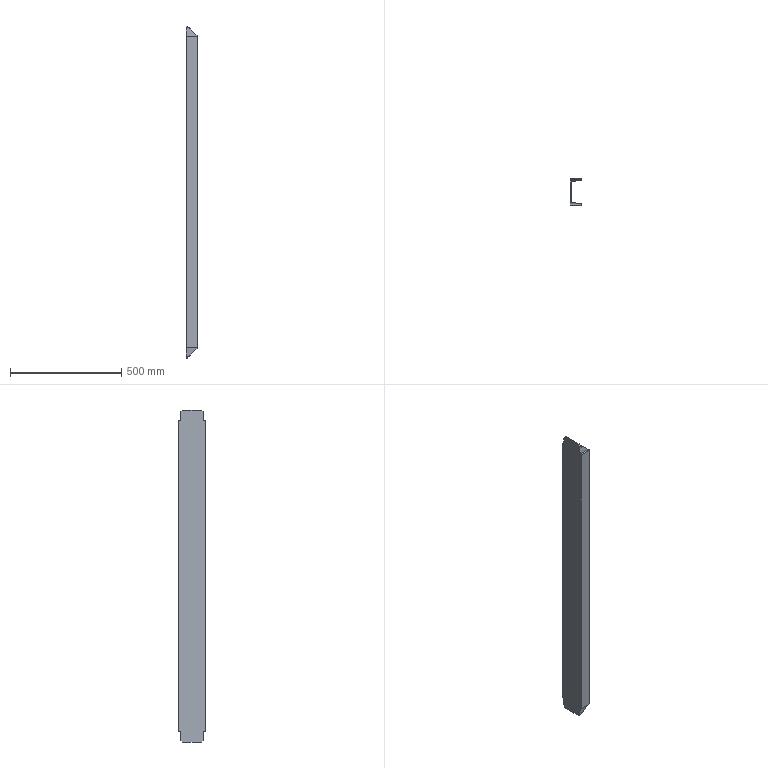Part | SolidWorks | features BaseBody 1 | 1 solid | 26 faces | box 53 x 120 x 1489 mm | volume 2202566 mm3 | plane 22 | cylinder 4 | commonest cylinder face diameters 9 x2 18 x2
STEP:
#1=CARTESIAN_POINT('',(13.559,49.351,536.441));
#2=VERTEX_POINT('',#1);
#3=CARTESIAN_POINT('',(0.,49.351,536.441));
#4=VERTEX_POINT('',#3);
#5=CARTESIAN_POINT('',(53.,49.351,536.441));
#6=DIRECTION('',(-1.,0.,0.));
#7=VECTOR('',#6,1000.);
#8=LINE('',#5,#7);
#9=EDGE_CURVE('',#2,#4,#8,.T.);
#10=ORIENTED_EDGE('',*,*,#9,.T.);
#11=CARTESIAN_POINT('',(0.,40.4,544.5));
#12=VERTEX_POINT('',#11);
#13=CARTESIAN_POINT('',(0.,40.4,544.5));
#14=DIRECTION('',(0.,-0.7431,0.6691));
#15=VECTOR('',#14,1000.);
#16=LINE('',#13,#15);
#17=EDGE_CURVE('',#4,#12,#16,.T.);
#18=ORIENTED_EDGE('',*,*,#17,.T.);
#19=CARTESIAN_POINT('',(5.5,40.4,544.5));
#20=VERTEX_POINT('',#19);
#21=CARTESIAN_POINT('',(48.5,40.4,544.5));
#22=DIRECTION('',(-1.,0.,0.));
#23=VECTOR('',#22,1000.);
#24=LINE('',#21,#23);
#25=EDGE_CURVE('',#20,#12,#24,.T.);
#26=ORIENTED_EDGE('',*,*,#25,.F.);
#27=CARTESIAN_POINT('',(13.559,49.351,536.441));
#28=CARTESIAN_POINT('',(8.741,48.844,536.897));
#29=CARTESIAN_POINT('',(5.5,45.244,540.138));
#30=CARTESIAN_POINT('',(5.5,40.4,544.5));
#31=(BOUNDED_CURVE()B_SPLINE_CURVE(3,(#27,#28,#29,#30),.UNSPECIFIED.,.F.,.F.)B_SPLINE_CURVE_WITH_KNOTS((4,4),(0.1047,1.571),.UNSPECIFIED.)CURVE()GEOMETRIC_REPRESENTATION_ITEM()RATIONAL_B_SPLINE_CURVE((1.,0.8288,0.8288,1.))REPRESENTATION_ITEM(''));
#32=EDGE_CURVE('',#2,#20,#31,.T.);
#33=ORIENTED_EDGE('',*,*,#32,.F.);
#34=EDGE_LOOP('',(#10,#18,#26,#33));
#35=FACE_OUTER_BOUND('',#34,.T.);
#36=CARTESIAN_POINT('',(53.,40.4,544.5));
#37=DIRECTION('',(0.,-0.6691,-0.7431));
#38=DIRECTION('',(0.,-0.7431,0.6691));
#39=AXIS2_PLACEMENT_3D('',#36,#37,#38);
#40=PLANE('',#39);
#41=ADVANCED_FACE('',(#35),#40,.F.);
#42=CARTESIAN_POINT('',(53.,60.,497.));
#43=VERTEX_POINT('',#42);
#44=CARTESIAN_POINT('',(53.,57.548,497.));
#45=VERTEX_POINT('',#44);
#46=CARTESIAN_POINT('',(53.,60.,497.));
#47=DIRECTION('',(0.,-1.,0.));
#48=VECTOR('',#47,1000.);
#49=LINE('',#46,#48);
#50=EDGE_CURVE('',#43,#45,#49,.T.);
#51=ORIENTED_EDGE('',*,*,#50,.F.);
#52=CARTESIAN_POINT('',(0.,60.,497.));
#53=VERTEX_POINT('',#52);
#54=CARTESIAN_POINT('',(53.,60.,497.));
#55=DIRECTION('',(-1.,0.,0.));
#56=VECTOR('',#55,1000.);
#57=LINE('',#54,#56);
#58=EDGE_CURVE('',#43,#53,#57,.T.);
#59=ORIENTED_EDGE('',*,*,#58,.T.);
#60=CARTESIAN_POINT('',(0.,53.496,497.));
#61=VERTEX_POINT('',#60);
#62=CARTESIAN_POINT('',(0.,60.,497.));
#63=DIRECTION('',(0.,-1.,0.));
#64=VECTOR('',#63,1000.);
#65=LINE('',#62,#64);
#66=EDGE_CURVE('',#53,#61,#65,.T.);
#67=ORIENTED_EDGE('',*,*,#66,.T.);
#68=CARTESIAN_POINT('',(50.458,53.496,497.));
#69=VERTEX_POINT('',#68);
#70=CARTESIAN_POINT('',(53.,53.496,497.));
#71=DIRECTION('',(-1.,0.,0.));
#72=VECTOR('',#71,1000.);
#73=LINE('',#70,#72);
#74=EDGE_CURVE('',#69,#61,#73,.T.);
#75=ORIENTED_EDGE('',*,*,#74,.F.);
#76=CARTESIAN_POINT('',(48.5,57.548,497.));
#77=DIRECTION('',(0.,0.,-1.));
#78=DIRECTION('',(0.,1.,0.));
#79=AXIS2_PLACEMENT_3D('',#76,#77,#78);
#80=CIRCLE('',#79,4.5);
#81=EDGE_CURVE('',#45,#69,#80,.T.);
#82=ORIENTED_EDGE('',*,*,#81,.F.);
#83=EDGE_LOOP('',(#51,#59,#67,#75,#82));
#84=FACE_OUTER_BOUND('',#83,.T.);
#85=CARTESIAN_POINT('',(53.,60.,497.));
#86=DIRECTION('',(0.,0.,-1.));
#87=DIRECTION('',(0.,-1.,0.));
#88=AXIS2_PLACEMENT_3D('',#85,#86,#87);
#89=PLANE('',#88);
#90=ADVANCED_FACE('',(#84),#89,.F.);
#91=CARTESIAN_POINT('',(48.97,53.073,501.03));
#92=VERTEX_POINT('',#91);
#93=CARTESIAN_POINT('',(50.458,53.496,497.));
#94=CARTESIAN_POINT('',(49.989,53.27,499.155));
#95=CARTESIAN_POINT('',(49.488,53.127,500.512));
#96=CARTESIAN_POINT('',(48.97,53.073,501.03));
#97=(BOUNDED_CURVE()B_SPLINE_CURVE(3,(#93,#94,#95,#96),.UNSPECIFIED.,.F.,.F.)B_SPLINE_CURVE_WITH_KNOTS((4,4),(2.691,3.037),.UNSPECIFIED.)CURVE()GEOMETRIC_REPRESENTATION_ITEM()RATIONAL_B_SPLINE_CURVE((1.,0.9901,0.9901,1.))REPRESENTATION_ITEM(''));
#98=EDGE_CURVE('',#69,#92,#97,.T.);
#99=ORIENTED_EDGE('',*,*,#98,.F.);
#100=ORIENTED_EDGE('',*,*,#74,.T.);
#101=CARTESIAN_POINT('',(0.,49.351,536.441));
#102=DIRECTION('',(0.,-0.1045,0.9945));
#103=VECTOR('',#102,1000.);
#104=LINE('',#101,#103);
#105=EDGE_CURVE('',#61,#4,#104,.T.);
#106=ORIENTED_EDGE('',*,*,#105,.T.);
#107=ORIENTED_EDGE('',*,*,#9,.F.);
#108=CARTESIAN_POINT('',(27.355,50.801,522.645));
#109=DIRECTION('',(-0.7052,-0.07412,0.7052));
#110=VECTOR('',#109,1000.);
#111=LINE('',#108,#110);
#112=EDGE_CURVE('',#92,#2,#111,.T.);
#113=ORIENTED_EDGE('',*,*,#112,.F.);
#114=EDGE_LOOP('',(#99,#100,#106,#107,#113));
#115=FACE_OUTER_BOUND('',#114,.T.);
#116=CARTESIAN_POINT('',(53.,49.351,536.441));
#117=DIRECTION('',(0.,-0.9945,-0.1045));
#118=DIRECTION('',(0.,0.1045,-0.9945));
#119=AXIS2_PLACEMENT_3D('',#116,#117,#118);
#120=PLANE('',#119);
#121=ADVANCED_FACE('',(#115),#120,.F.);
#122=CARTESIAN_POINT('',(0.,-40.4,544.5));
#123=VERTEX_POINT('',#122);
#124=CARTESIAN_POINT('',(5.5,-40.4,544.5));
#125=VERTEX_POINT('',#124);
#126=CARTESIAN_POINT('',(48.5,-40.4,544.5));
#127=DIRECTION('',(1.,0.,0.));
#128=VECTOR('',#127,1000.);
#129=LINE('',#126,#128);
#130=EDGE_CURVE('',#123,#125,#129,.T.);
#131=ORIENTED_EDGE('',*,*,#130,.F.);
#132=CARTESIAN_POINT('',(0.,-49.351,536.441));
#133=VERTEX_POINT('',#132);
#134=CARTESIAN_POINT('',(0.,-40.4,544.5));
#135=DIRECTION('',(0.,-0.7431,-0.6691));
#136=VECTOR('',#135,1000.);
#137=LINE('',#134,#136);
#138=EDGE_CURVE('',#123,#133,#137,.T.);
#139=ORIENTED_EDGE('',*,*,#138,.T.);
#140=CARTESIAN_POINT('',(13.559,-49.351,536.441));
#141=VERTEX_POINT('',#140);
#142=CARTESIAN_POINT('',(53.,-49.351,536.441));
#143=DIRECTION('',(-1.,0.,0.));
#144=VECTOR('',#143,1000.);
#145=LINE('',#142,#144);
#146=EDGE_CURVE('',#141,#133,#145,.T.);
#147=ORIENTED_EDGE('',*,*,#146,.F.);
#148=CARTESIAN_POINT('',(5.5,-40.4,544.5));
#149=CARTESIAN_POINT('',(5.5,-45.244,540.138));
#150=CARTESIAN_POINT('',(8.741,-48.844,536.897));
#151=CARTESIAN_POINT('',(13.559,-49.351,536.441));
#152=(BOUNDED_CURVE()B_SPLINE_CURVE(3,(#148,#149,#150,#151),.UNSPECIFIED.,.F.,.F.)B_SPLINE_CURVE_WITH_KNOTS((4,4),(4.712,6.178),.UNSPECIFIED.)CURVE()GEOMETRIC_REPRESENTATION_ITEM()RATIONAL_B_SPLINE_CURVE((1.,0.8288,0.8288,1.))REPRESENTATION_ITEM(''));
#153=EDGE_CURVE('',#125,#141,#152,.T.);
#154=ORIENTED_EDGE('',*,*,#153,.F.);
#155=EDGE_LOOP('',(#131,#139,#147,#154));
#156=FACE_OUTER_BOUND('',#155,.T.);
#157=CARTESIAN_POINT('',(53.,-40.4,544.5));
#158=DIRECTION('',(0.,0.6691,-0.7431));
#159=DIRECTION('',(-1.,0.,0.));
#160=AXIS2_PLACEMENT_3D('',#157,#158,#159);
#161=PLANE('',#160);
#162=ADVANCED_FACE('',(#156),#161,.F.);
#163=CARTESIAN_POINT('',(48.97,-53.073,501.03));
#164=VERTEX_POINT('',#163);
#165=CARTESIAN_POINT('',(27.355,-50.801,522.645));
#166=DIRECTION('',(0.7052,-0.07412,-0.7052));
#167=VECTOR('',#166,1000.);
#168=LINE('',#165,#167);
#169=EDGE_CURVE('',#141,#164,#168,.T.);
#170=ORIENTED_EDGE('',*,*,#169,.F.);
#171=ORIENTED_EDGE('',*,*,#146,.T.);
#172=CARTESIAN_POINT('',(0.,-53.496,497.));
#173=VERTEX_POINT('',#172);
#174=CARTESIAN_POINT('',(0.,-49.351,536.441));
#175=DIRECTION('',(0.,-0.1045,-0.9945));
#176=VECTOR('',#175,1000.);
#177=LINE('',#174,#176);
#178=EDGE_CURVE('',#133,#173,#177,.T.);
#179=ORIENTED_EDGE('',*,*,#178,.T.);
#180=CARTESIAN_POINT('',(50.458,-53.496,497.));
#181=VERTEX_POINT('',#180);
#182=CARTESIAN_POINT('',(53.,-53.496,497.));
#183=DIRECTION('',(-1.,0.,0.));
#184=VECTOR('',#183,1000.);
#185=LINE('',#182,#184);
#186=EDGE_CURVE('',#181,#173,#185,.T.);
#187=ORIENTED_EDGE('',*,*,#186,.F.);
#188=CARTESIAN_POINT('',(48.97,-53.073,501.03));
#189=CARTESIAN_POINT('',(49.488,-53.127,500.512));
#190=CARTESIAN_POINT('',(49.989,-53.27,499.155));
#191=CARTESIAN_POINT('',(50.458,-53.496,497.));
#192=(BOUNDED_CURVE()B_SPLINE_CURVE(3,(#188,#189,#190,#191),.UNSPECIFIED.,.F.,.F.)B_SPLINE_CURVE_WITH_KNOTS((4,4),(3.246,3.592),.UNSPECIFIED.)CURVE()GEOMETRIC_REPRESENTATION_ITEM()RATIONAL_B_SPLINE_CURVE((1.,0.9901,0.9901,1.))REPRESENTATION_ITEM(''));
#193=EDGE_CURVE('',#164,#181,#192,.T.);
#194=ORIENTED_EDGE('',*,*,#193,.F.);
#195=EDGE_LOOP('',(#170,#171,#179,#187,#194));
#196=FACE_OUTER_BOUND('',#195,.T.);
#197=CARTESIAN_POINT('',(53.,-49.351,536.441));
#198=DIRECTION('',(0.,0.9945,-0.1045));
#199=DIRECTION('',(-1.,0.,0.));
#200=AXIS2_PLACEMENT_3D('',#197,#198,#199);
#201=PLANE('',#200);
#202=ADVANCED_FACE('',(#196),#201,.F.);
#203=ORIENTED_EDGE('',*,*,#186,.T.);
#204=CARTESIAN_POINT('',(0.,-60.,497.));
#205=VERTEX_POINT('',#204);
#206=CARTESIAN_POINT('',(0.,-60.,497.));
#207=DIRECTION('',(0.,-1.,0.));
#208=VECTOR('',#207,1000.);
#209=LINE('',#206,#208);
#210=EDGE_CURVE('',#173,#205,#209,.T.);
#211=ORIENTED_EDGE('',*,*,#210,.T.);
#212=CARTESIAN_POINT('',(53.,-60.,497.));
#213=VERTEX_POINT('',#212);
#214=CARTESIAN_POINT('',(53.,-60.,497.));
#215=DIRECTION('',(-1.,0.,0.));
#216=VECTOR('',#215,1000.);
#217=LINE('',#214,#216);
#218=EDGE_CURVE('',#213,#205,#217,.T.);
#219=ORIENTED_EDGE('',*,*,#218,.F.);
#220=CARTESIAN_POINT('',(53.,-57.548,497.));
#221=VERTEX_POINT('',#220);
#222=CARTESIAN_POINT('',(53.,-60.,497.));
#223=DIRECTION('',(0.,-1.,0.));
#224=VECTOR('',#223,1000.);
#225=LINE('',#222,#224);
#226=EDGE_CURVE('',#221,#213,#225,.T.);
#227=ORIENTED_EDGE('',*,*,#226,.F.);
#228=CARTESIAN_POINT('',(48.5,-57.548,497.));
#229=DIRECTION('',(0.,0.,-1.));
#230=DIRECTION('',(0.,1.,0.));
#231=AXIS2_PLACEMENT_3D('',#228,#229,#230);
#232=CIRCLE('',#231,4.5);
#233=EDGE_CURVE('',#181,#221,#232,.T.);
#234=ORIENTED_EDGE('',*,*,#233,.F.);
#235=EDGE_LOOP('',(#203,#211,#219,#227,#234));
#236=FACE_OUTER_BOUND('',#235,.T.);
#237=CARTESIAN_POINT('',(53.,-60.,497.));
#238=DIRECTION('',(0.,0.,-1.));
#239=DIRECTION('',(-1.,0.,0.));
#240=AXIS2_PLACEMENT_3D('',#237,#238,#239);
#241=PLANE('',#240);
#242=ADVANCED_FACE('',(#236),#241,.F.);
#243=CARTESIAN_POINT('',(13.559,-49.351,-936.441));
#244=VERTEX_POINT('',#243);
#245=CARTESIAN_POINT('',(0.,-49.351,-936.441));
#246=VERTEX_POINT('',#245);
#247=CARTESIAN_POINT('',(53.,-49.351,-936.441));
#248=DIRECTION('',(-1.,0.,0.));
#249=VECTOR('',#248,1000.);
#250=LINE('',#247,#249);
#251=EDGE_CURVE('',#244,#246,#250,.T.);
#252=ORIENTED_EDGE('',*,*,#251,.T.);
#253=CARTESIAN_POINT('',(0.,-40.4,-944.5));
#254=VERTEX_POINT('',#253);
#255=CARTESIAN_POINT('',(0.,-40.4,-944.5));
#256=DIRECTION('',(0.,0.7431,-0.6691));
#257=VECTOR('',#256,1000.);
#258=LINE('',#255,#257);
#259=EDGE_CURVE('',#246,#254,#258,.T.);
#260=ORIENTED_EDGE('',*,*,#259,.T.);
#261=CARTESIAN_POINT('',(5.5,-40.4,-944.5));
#262=VERTEX_POINT('',#261);
#263=CARTESIAN_POINT('',(48.5,-40.4,-944.5));
#264=DIRECTION('',(1.,0.,0.));
#265=VECTOR('',#264,1000.);
#266=LINE('',#263,#265);
#267=EDGE_CURVE('',#254,#262,#266,.T.);
#268=ORIENTED_EDGE('',*,*,#267,.T.);
#269=CARTESIAN_POINT('',(13.559,-49.351,-936.441));
#270=CARTESIAN_POINT('',(8.741,-48.844,-936.897));
#271=CARTESIAN_POINT('',(5.5,-45.244,-940.138));
#272=CARTESIAN_POINT('',(5.5,-40.4,-944.5));
#273=(BOUNDED_CURVE()B_SPLINE_CURVE(3,(#269,#270,#271,#272),.UNSPECIFIED.,.F.,.F.)B_SPLINE_CURVE_WITH_KNOTS((4,4),(3.246,4.712),.UNSPECIFIED.)CURVE()GEOMETRIC_REPRESENTATION_ITEM()RATIONAL_B_SPLINE_CURVE((1.,0.8288,0.8288,1.))REPRESENTATION_ITEM(''));
#274=EDGE_CURVE('',#244,#262,#273,.T.);
#275=ORIENTED_EDGE('',*,*,#274,.F.);
#276=EDGE_LOOP('',(#252,#260,#268,#275));
#277=FACE_OUTER_BOUND('',#276,.T.);
#278=CARTESIAN_POINT('',(53.,-40.4,-944.5));
#279=DIRECTION('',(0.,0.6691,0.7431));
#280=DIRECTION('',(1.,0.,0.));
#281=AXIS2_PLACEMENT_3D('',#278,#279,#280);
#282=PLANE('',#281);
#283=ADVANCED_FACE('',(#277),#282,.F.);
#284=CARTESIAN_POINT('',(50.458,-53.496,-897.));
#285=VERTEX_POINT('',#284);
#286=CARTESIAN_POINT('',(0.,-53.496,-897.));
#287=VERTEX_POINT('',#286);
#288=CARTESIAN_POINT('',(53.,-53.496,-897.));
#289=DIRECTION('',(-1.,0.,0.));
#290=VECTOR('',#289,1000.);
#291=LINE('',#288,#290);
#292=EDGE_CURVE('',#285,#287,#291,.T.);
#293=ORIENTED_EDGE('',*,*,#292,.T.);
#294=CARTESIAN_POINT('',(0.,-49.351,-936.441));
#295=DIRECTION('',(0.,0.1045,-0.9945));
#296=VECTOR('',#295,1000.);
#297=LINE('',#294,#296);
#298=EDGE_CURVE('',#287,#246,#297,.T.);
#299=ORIENTED_EDGE('',*,*,#298,.T.);
#300=ORIENTED_EDGE('',*,*,#251,.F.);
#301=CARTESIAN_POINT('',(48.97,-53.073,-901.03));
#302=VERTEX_POINT('',#301);
#303=CARTESIAN_POINT('',(568.864,-107.716,-381.136));
#304=DIRECTION('',(-0.7052,0.07412,-0.7052));
#305=VECTOR('',#304,1000.);
#306=LINE('',#303,#305);
#307=EDGE_CURVE('',#302,#244,#306,.T.);
#308=ORIENTED_EDGE('',*,*,#307,.F.);
#309=CARTESIAN_POINT('',(50.458,-53.496,-897.));
#310=CARTESIAN_POINT('',(49.989,-53.27,-899.155));
#311=CARTESIAN_POINT('',(49.488,-53.127,-900.512));
#312=CARTESIAN_POINT('',(48.97,-53.073,-901.03));
#313=(BOUNDED_CURVE()B_SPLINE_CURVE(3,(#309,#310,#311,#312),.UNSPECIFIED.,.F.,.F.)B_SPLINE_CURVE_WITH_KNOTS((4,4),(5.833,6.178),.UNSPECIFIED.)CURVE()GEOMETRIC_REPRESENTATION_ITEM()RATIONAL_B_SPLINE_CURVE((1.,0.9901,0.9901,1.))REPRESENTATION_ITEM(''));
#314=EDGE_CURVE('',#285,#302,#313,.T.);
#315=ORIENTED_EDGE('',*,*,#314,.F.);
#316=EDGE_LOOP('',(#293,#299,#300,#308,#315));
#317=FACE_OUTER_BOUND('',#316,.T.);
#318=CARTESIAN_POINT('',(53.,-49.351,-936.441));
#319=DIRECTION('',(0.,0.9945,0.1045));
#320=DIRECTION('',(1.,0.,0.));
#321=AXIS2_PLACEMENT_3D('',#318,#319,#320);
#322=PLANE('',#321);
#323=ADVANCED_FACE('',(#317),#322,.F.);
#324=CARTESIAN_POINT('',(53.,-60.,-897.));
#325=VERTEX_POINT('',#324);
#326=CARTESIAN_POINT('',(53.,-57.548,-897.));
#327=VERTEX_POINT('',#326);
#328=CARTESIAN_POINT('',(53.,-60.,-897.));
#329=DIRECTION('',(0.,1.,0.));
#330=VECTOR('',#329,1000.);
#331=LINE('',#328,#330);
#332=EDGE_CURVE('',#325,#327,#331,.T.);
#333=ORIENTED_EDGE('',*,*,#332,.F.);
#334=CARTESIAN_POINT('',(0.,-60.,-897.));
#335=VERTEX_POINT('',#334);
#336=CARTESIAN_POINT('',(53.,-60.,-897.));
#337=DIRECTION('',(-1.,0.,0.));
#338=VECTOR('',#337,1000.);
#339=LINE('',#336,#338);
#340=EDGE_CURVE('',#325,#335,#339,.T.);
#341=ORIENTED_EDGE('',*,*,#340,.T.);
#342=CARTESIAN_POINT('',(0.,-60.,-897.));
#343=DIRECTION('',(0.,1.,0.));
#344=VECTOR('',#343,1000.);
#345=LINE('',#342,#344);
#346=EDGE_CURVE('',#335,#287,#345,.T.);
#347=ORIENTED_EDGE('',*,*,#346,.T.);
#348=ORIENTED_EDGE('',*,*,#292,.F.);
#349=CARTESIAN_POINT('',(48.5,-57.548,-897.));
#350=DIRECTION('',(0.,0.,1.));
#351=DIRECTION('',(0.,-1.,0.));
#352=AXIS2_PLACEMENT_3D('',#349,#350,#351);
#353=CIRCLE('',#352,4.5);
#354=EDGE_CURVE('',#327,#285,#353,.T.);
#355=ORIENTED_EDGE('',*,*,#354,.F.);
#356=EDGE_LOOP('',(#333,#341,#347,#348,#355));
#357=FACE_OUTER_BOUND('',#356,.T.);
#358=CARTESIAN_POINT('',(53.,-60.,-897.));
#359=DIRECTION('',(0.,0.,1.));
#360=DIRECTION('',(0.,-1.,0.));
#361=AXIS2_PLACEMENT_3D('',#358,#359,#360);
#362=PLANE('',#361);
#363=ADVANCED_FACE('',(#357),#362,.F.);
#364=CARTESIAN_POINT('',(5.5,40.4,-944.5));
#365=VERTEX_POINT('',#364);
#366=CARTESIAN_POINT('',(0.,40.4,-944.5));
#367=VERTEX_POINT('',#366);
#368=CARTESIAN_POINT('',(48.5,40.4,-944.5));
#369=DIRECTION('',(-1.,0.,0.));
#370=VECTOR('',#369,1000.);
#371=LINE('',#368,#370);
#372=EDGE_CURVE('',#365,#367,#371,.T.);
#373=ORIENTED_EDGE('',*,*,#372,.T.);
#374=CARTESIAN_POINT('',(0.,49.351,-936.441));
#375=VERTEX_POINT('',#374);
#376=CARTESIAN_POINT('',(0.,40.4,-944.5));
#377=DIRECTION('',(0.,0.7431,0.6691));
#378=VECTOR('',#377,1000.);
#379=LINE('',#376,#378);
#380=EDGE_CURVE('',#367,#375,#379,.T.);
#381=ORIENTED_EDGE('',*,*,#380,.T.);
#382=CARTESIAN_POINT('',(13.559,49.351,-936.441));
#383=VERTEX_POINT('',#382);
#384=CARTESIAN_POINT('',(53.,49.351,-936.441));
#385=DIRECTION('',(-1.,0.,0.));
#386=VECTOR('',#385,1000.);
#387=LINE('',#384,#386);
#388=EDGE_CURVE('',#383,#375,#387,.T.);
#389=ORIENTED_EDGE('',*,*,#388,.F.);
#390=CARTESIAN_POINT('',(5.5,40.4,-944.5));
#391=CARTESIAN_POINT('',(5.5,45.244,-940.138));
#392=CARTESIAN_POINT('',(8.741,48.844,-936.897));
#393=CARTESIAN_POINT('',(13.559,49.351,-936.441));
#394=(BOUNDED_CURVE()B_SPLINE_CURVE(3,(#390,#391,#392,#393),.UNSPECIFIED.,.F.,.F.)B_SPLINE_CURVE_WITH_KNOTS((4,4),(1.571,3.037),.UNSPECIFIED.)CURVE()GEOMETRIC_REPRESENTATION_ITEM()RATIONAL_B_SPLINE_CURVE((1.,0.8288,0.8288,1.))REPRESENTATION_ITEM(''));
#395=EDGE_CURVE('',#365,#383,#394,.T.);
#396=ORIENTED_EDGE('',*,*,#395,.F.);
#397=EDGE_LOOP('',(#373,#381,#389,#396));
#398=FACE_OUTER_BOUND('',#397,.T.);
#399=CARTESIAN_POINT('',(53.,40.4,-944.5));
#400=DIRECTION('',(0.,-0.6691,0.7431));
#401=DIRECTION('',(-1.,0.,0.));
#402=AXIS2_PLACEMENT_3D('',#399,#400,#401);
#403=PLANE('',#402);
#404=ADVANCED_FACE('',(#398),#403,.F.);
#405=CARTESIAN_POINT('',(50.458,53.496,-897.));
#406=VERTEX_POINT('',#405);
#407=CARTESIAN_POINT('',(0.,53.496,-897.));
#408=VERTEX_POINT('',#407);
#409=CARTESIAN_POINT('',(53.,53.496,-897.));
#410=DIRECTION('',(-1.,0.,0.));
#411=VECTOR('',#410,1000.);
#412=LINE('',#409,#411);
#413=EDGE_CURVE('',#406,#408,#412,.T.);
#414=ORIENTED_EDGE('',*,*,#413,.T.);
#415=CARTESIAN_POINT('',(0.,60.,-897.));
#416=VERTEX_POINT('',#415);
#417=CARTESIAN_POINT('',(0.,60.,-897.));
#418=DIRECTION('',(0.,1.,0.));
#419=VECTOR('',#418,1000.);
#420=LINE('',#417,#419);
#421=EDGE_CURVE('',#408,#416,#420,.T.);
#422=ORIENTED_EDGE('',*,*,#421,.T.);
#423=CARTESIAN_POINT('',(53.,60.,-897.));
#424=VERTEX_POINT('',#423);
#425=CARTESIAN_POINT('',(53.,60.,-897.));
#426=DIRECTION('',(-1.,0.,0.));
#427=VECTOR('',#426,1000.);
#428=LINE('',#425,#427);
#429=EDGE_CURVE('',#424,#416,#428,.T.);
#430=ORIENTED_EDGE('',*,*,#429,.F.);
#431=CARTESIAN_POINT('',(53.,57.548,-897.));
#432=VERTEX_POINT('',#431);
#433=CARTESIAN_POINT('',(53.,60.,-897.));
#434=DIRECTION('',(0.,1.,0.));
#435=VECTOR('',#434,1000.);
#436=LINE('',#433,#435);
#437=EDGE_CURVE('',#432,#424,#436,.T.);
#438=ORIENTED_EDGE('',*,*,#437,.F.);
#439=CARTESIAN_POINT('',(48.5,57.548,-897.));
#440=DIRECTION('',(0.,0.,1.));
#441=DIRECTION('',(0.,-1.,0.));
#442=AXIS2_PLACEMENT_3D('',#439,#440,#441);
#443=CIRCLE('',#442,4.5);
#444=EDGE_CURVE('',#406,#432,#443,.T.);
#445=ORIENTED_EDGE('',*,*,#444,.F.);
#446=EDGE_LOOP('',(#414,#422,#430,#438,#445));
#447=FACE_OUTER_BOUND('',#446,.T.);
#448=CARTESIAN_POINT('',(53.,60.,-897.));
#449=DIRECTION('',(0.,0.,1.));
#450=DIRECTION('',(0.,-1.,0.));
#451=AXIS2_PLACEMENT_3D('',#448,#449,#450);
#452=PLANE('',#451);
#453=ADVANCED_FACE('',(#447),#452,.F.);
#454=ORIENTED_EDGE('',*,*,#388,.T.);
#455=CARTESIAN_POINT('',(0.,49.351,-936.441));
#456=DIRECTION('',(0.,0.1045,0.9945));
#457=VECTOR('',#456,1000.);
#458=LINE('',#455,#457);
#459=EDGE_CURVE('',#375,#408,#458,.T.);
#460=ORIENTED_EDGE('',*,*,#459,.T.);
#461=ORIENTED_EDGE('',*,*,#413,.F.);
#462=CARTESIAN_POINT('',(48.97,53.073,-901.03));
#463=VERTEX_POINT('',#462);
#464=CARTESIAN_POINT('',(48.97,53.073,-901.03));
#465=CARTESIAN_POINT('',(49.488,53.127,-900.512));
#466=CARTESIAN_POINT('',(49.989,53.27,-899.155));
#467=CARTESIAN_POINT('',(50.458,53.496,-897.));
#468=(BOUNDED_CURVE()B_SPLINE_CURVE(3,(#464,#465,#466,#467),.UNSPECIFIED.,.F.,.F.)B_SPLINE_CURVE_WITH_KNOTS((4,4),(0.1047,0.4501),.UNSPECIFIED.)CURVE()GEOMETRIC_REPRESENTATION_ITEM()RATIONAL_B_SPLINE_CURVE((1.,0.9901,0.9901,1.))REPRESENTATION_ITEM(''));
#469=EDGE_CURVE('',#463,#406,#468,.T.);
#470=ORIENTED_EDGE('',*,*,#469,.F.);
#471=CARTESIAN_POINT('',(568.864,107.716,-381.136));
#472=DIRECTION('',(0.7052,0.07412,0.7052));
#473=VECTOR('',#472,1000.);
#474=LINE('',#471,#473);
#475=EDGE_CURVE('',#383,#463,#474,.T.);
#476=ORIENTED_EDGE('',*,*,#475,.F.);
#477=EDGE_LOOP('',(#454,#460,#461,#470,#476));
#478=FACE_OUTER_BOUND('',#477,.T.);
#479=CARTESIAN_POINT('',(53.,49.351,-936.441));
#480=DIRECTION('',(0.,-0.9945,0.1045));
#481=DIRECTION('',(-1.,0.,0.));
#482=AXIS2_PLACEMENT_3D('',#479,#480,#481);
#483=PLANE('',#482);
#484=ADVANCED_FACE('',(#478),#483,.F.);
#485=ORIENTED_EDGE('',*,*,#267,.F.);
#486=CARTESIAN_POINT('',(0.,-60.,-944.5));
#487=DIRECTION('',(0.,-1.,0.));
#488=VECTOR('',#487,1000.);
#489=LINE('',#486,#488);
#490=EDGE_CURVE('',#367,#254,#489,.T.);
#491=ORIENTED_EDGE('',*,*,#490,.F.);
#492=ORIENTED_EDGE('',*,*,#372,.F.);
#493=CARTESIAN_POINT('',(5.5,-40.4,-944.5));
#494=DIRECTION('',(0.,1.,0.));
#495=VECTOR('',#494,1000.);
#496=LINE('',#493,#495);
#497=EDGE_CURVE('',#262,#365,#496,.T.);
#498=ORIENTED_EDGE('',*,*,#497,.F.);
#499=EDGE_LOOP('',(#485,#491,#492,#498));
#500=FACE_OUTER_BOUND('',#499,.T.);
#501=CARTESIAN_POINT('',(48.5,57.548,-944.5));
#502=DIRECTION('',(0.,0.,-1.));
#503=DIRECTION('',(0.,-1.,0.));
#504=AXIS2_PLACEMENT_3D('',#501,#502,#503);
#505=PLANE('',#504);
#506=ADVANCED_FACE('',(#500),#505,.T.);
#507=CARTESIAN_POINT('',(5.5,-40.4,544.5));
#508=DIRECTION('',(0.,1.,0.));
#509=VECTOR('',#508,1000.);
#510=LINE('',#507,#509);
#511=EDGE_CURVE('',#125,#20,#510,.T.);
#512=ORIENTED_EDGE('',*,*,#511,.T.);
#513=ORIENTED_EDGE('',*,*,#25,.T.);
#514=CARTESIAN_POINT('',(0.,-60.,544.5));
#515=DIRECTION('',(0.,-1.,0.));
#516=VECTOR('',#515,1000.);
#517=LINE('',#514,#516);
#518=EDGE_CURVE('',#12,#123,#517,.T.);
#519=ORIENTED_EDGE('',*,*,#518,.T.);
#520=ORIENTED_EDGE('',*,*,#130,.T.);
#521=EDGE_LOOP('',(#512,#513,#519,#520));
#522=FACE_OUTER_BOUND('',#521,.T.);
#523=CARTESIAN_POINT('',(48.5,57.548,544.5));
#524=DIRECTION('',(0.,0.,-1.));
#525=DIRECTION('',(0.,-1.,0.));
#526=AXIS2_PLACEMENT_3D('',#523,#524,#525);
#527=PLANE('',#526);
#528=ADVANCED_FACE('',(#522),#527,.F.);
#529=CARTESIAN_POINT('',(53.,60.,544.5));
#530=DIRECTION('',(0.,0.,-1.));
#531=VECTOR('',#530,1000.);
#532=LINE('',#529,#531);
#533=EDGE_CURVE('',#43,#424,#532,.T.);
#534=ORIENTED_EDGE('',*,*,#533,.F.);
#535=ORIENTED_EDGE('',*,*,#50,.T.);
#536=CARTESIAN_POINT('',(53.,57.548,544.5));
#537=DIRECTION('',(0.,0.,-1.));
#538=VECTOR('',#537,1000.);
#539=LINE('',#536,#538);
#540=EDGE_CURVE('',#45,#432,#539,.T.);
#541=ORIENTED_EDGE('',*,*,#540,.T.);
#542=ORIENTED_EDGE('',*,*,#437,.T.);
#543=EDGE_LOOP('',(#534,#535,#541,#542));
#544=FACE_OUTER_BOUND('',#543,.T.);
#545=CARTESIAN_POINT('',(53.,60.,544.5));
#546=DIRECTION('',(-1.,0.,0.));
#547=DIRECTION('',(0.,0.,1.));
#548=AXIS2_PLACEMENT_3D('',#545,#546,#547);
#549=PLANE('',#548);
#550=ADVANCED_FACE('',(#544),#549,.F.);
#551=ORIENTED_EDGE('',*,*,#81,.T.);
#552=ORIENTED_EDGE('',*,*,#98,.T.);
#553=CARTESIAN_POINT('',(48.97,53.073,544.5));
#554=DIRECTION('',(0.,0.,-1.));
#555=VECTOR('',#554,1000.);
#556=LINE('',#553,#555);
#557=EDGE_CURVE('',#92,#463,#556,.T.);
#558=ORIENTED_EDGE('',*,*,#557,.T.);
#559=ORIENTED_EDGE('',*,*,#469,.T.);
#560=ORIENTED_EDGE('',*,*,#444,.T.);
#561=ORIENTED_EDGE('',*,*,#540,.F.);
#562=EDGE_LOOP('',(#551,#552,#558,#559,#560,#561));
#563=FACE_OUTER_BOUND('',#562,.T.);
#564=CARTESIAN_POINT('',(48.5,57.548,544.5));
#565=DIRECTION('',(0.,0.,-1.));
#566=DIRECTION('',(-1.,0.,0.));
#567=AXIS2_PLACEMENT_3D('',#564,#565,#566);
#568=CYLINDRICAL_SURFACE('',#567,4.5);
#569=ADVANCED_FACE('',(#563),#568,.T.);
#570=ORIENTED_EDGE('',*,*,#557,.F.);
#571=ORIENTED_EDGE('',*,*,#112,.T.);
#572=CARTESIAN_POINT('',(13.559,49.351,544.5));
#573=DIRECTION('',(0.,0.,-1.));
#574=VECTOR('',#573,1000.);
#575=LINE('',#572,#574);
#576=EDGE_CURVE('',#2,#383,#575,.T.);
#577=ORIENTED_EDGE('',*,*,#576,.T.);
#578=ORIENTED_EDGE('',*,*,#475,.T.);
#579=EDGE_LOOP('',(#570,#571,#577,#578));
#580=FACE_OUTER_BOUND('',#579,.T.);
#581=CARTESIAN_POINT('',(48.97,53.073,544.5));
#582=DIRECTION('',(-0.1045,0.9945,0.));
#583=DIRECTION('',(0.,0.,1.));
#584=AXIS2_PLACEMENT_3D('',#581,#582,#583);
#585=PLANE('',#584);
#586=ADVANCED_FACE('',(#580),#585,.F.);
#587=ORIENTED_EDGE('',*,*,#576,.F.);
#588=ORIENTED_EDGE('',*,*,#32,.T.);
#589=CARTESIAN_POINT('',(5.5,40.4,544.5));
#590=DIRECTION('',(0.,0.,-1.));
#591=VECTOR('',#590,1000.);
#592=LINE('',#589,#591);
#593=EDGE_CURVE('',#20,#365,#592,.T.);
#594=ORIENTED_EDGE('',*,*,#593,.T.);
#595=ORIENTED_EDGE('',*,*,#395,.T.);
#596=EDGE_LOOP('',(#587,#588,#594,#595));
#597=FACE_OUTER_BOUND('',#596,.T.);
#598=CARTESIAN_POINT('',(14.5,40.4,544.5));
#599=DIRECTION('',(0.,0.,-1.));
#600=DIRECTION('',(-1.,0.,0.));
#601=AXIS2_PLACEMENT_3D('',#598,#599,#600);
#602=CYLINDRICAL_SURFACE('',#601,9.);
#603=ADVANCED_FACE('',(#597),#602,.F.);
#604=ORIENTED_EDGE('',*,*,#497,.T.);
#605=ORIENTED_EDGE('',*,*,#593,.F.);
#606=ORIENTED_EDGE('',*,*,#511,.F.);
#607=CARTESIAN_POINT('',(5.5,-40.4,544.5));
#608=DIRECTION('',(0.,0.,-1.));
#609=VECTOR('',#608,1000.);
#610=LINE('',#607,#609);
#611=EDGE_CURVE('',#125,#262,#610,.T.);
#612=ORIENTED_EDGE('',*,*,#611,.T.);
#613=EDGE_LOOP('',(#604,#605,#606,#612));
#614=FACE_OUTER_BOUND('',#613,.T.);
#615=CARTESIAN_POINT('',(5.5,-40.4,544.5));
#616=DIRECTION('',(-1.,0.,0.));
#617=DIRECTION('',(0.,1.,0.));
#618=AXIS2_PLACEMENT_3D('',#615,#616,#617);
#619=PLANE('',#618);
#620=ADVANCED_FACE('',(#614),#619,.F.);
#621=ORIENTED_EDGE('',*,*,#611,.F.);
#622=ORIENTED_EDGE('',*,*,#153,.T.);
#623=CARTESIAN_POINT('',(13.559,-49.351,544.5));
#624=DIRECTION('',(0.,0.,-1.));
#625=VECTOR('',#624,1000.);
#626=LINE('',#623,#625);
#627=EDGE_CURVE('',#141,#244,#626,.T.);
#628=ORIENTED_EDGE('',*,*,#627,.T.);
#629=ORIENTED_EDGE('',*,*,#274,.T.);
#630=EDGE_LOOP('',(#621,#622,#628,#629));
#631=FACE_OUTER_BOUND('',#630,.T.);
#632=CARTESIAN_POINT('',(14.5,-40.4,544.5));
#633=DIRECTION('',(0.,0.,-1.));
#634=DIRECTION('',(-1.,0.,0.));
#635=AXIS2_PLACEMENT_3D('',#632,#633,#634);
#636=CYLINDRICAL_SURFACE('',#635,9.);
#637=ADVANCED_FACE('',(#631),#636,.F.);
#638=ORIENTED_EDGE('',*,*,#627,.F.);
#639=ORIENTED_EDGE('',*,*,#169,.T.);
#640=CARTESIAN_POINT('',(48.97,-53.073,544.5));
#641=DIRECTION('',(0.,0.,-1.));
#642=VECTOR('',#641,1000.);
#643=LINE('',#640,#642);
#644=EDGE_CURVE('',#164,#302,#643,.T.);
#645=ORIENTED_EDGE('',*,*,#644,.T.);
#646=ORIENTED_EDGE('',*,*,#307,.T.);
#647=EDGE_LOOP('',(#638,#639,#645,#646));
#648=FACE_OUTER_BOUND('',#647,.T.);
#649=CARTESIAN_POINT('',(48.97,-53.073,544.5));
#650=DIRECTION('',(-0.1045,-0.9945,0.));
#651=DIRECTION('',(-0.9945,0.1045,0.));
#652=AXIS2_PLACEMENT_3D('',#649,#650,#651);
#653=PLANE('',#652);
#654=ADVANCED_FACE('',(#648),#653,.F.);
#655=ORIENTED_EDGE('',*,*,#193,.T.);
#656=ORIENTED_EDGE('',*,*,#233,.T.);
#657=CARTESIAN_POINT('',(53.,-57.548,544.5));
#658=DIRECTION('',(0.,0.,-1.));
#659=VECTOR('',#658,1000.);
#660=LINE('',#657,#659);
#661=EDGE_CURVE('',#221,#327,#660,.T.);
#662=ORIENTED_EDGE('',*,*,#661,.T.);
#663=ORIENTED_EDGE('',*,*,#354,.T.);
#664=ORIENTED_EDGE('',*,*,#314,.T.);
#665=ORIENTED_EDGE('',*,*,#644,.F.);
#666=EDGE_LOOP('',(#655,#656,#662,#663,#664,#665));
#667=FACE_OUTER_BOUND('',#666,.T.);
#668=CARTESIAN_POINT('',(48.5,-57.548,544.5));
#669=DIRECTION('',(0.,0.,-1.));
#670=DIRECTION('',(-1.,0.,0.));
#671=AXIS2_PLACEMENT_3D('',#668,#669,#670);
#672=CYLINDRICAL_SURFACE('',#671,4.5);
#673=ADVANCED_FACE('',(#667),#672,.T.);
#674=ORIENTED_EDGE('',*,*,#661,.F.);
#675=ORIENTED_EDGE('',*,*,#226,.T.);
#676=CARTESIAN_POINT('',(53.,-60.,544.5));
#677=DIRECTION('',(0.,0.,-1.));
#678=VECTOR('',#677,1000.);
#679=LINE('',#676,#678);
#680=EDGE_CURVE('',#213,#325,#679,.T.);
#681=ORIENTED_EDGE('',*,*,#680,.T.);
#682=ORIENTED_EDGE('',*,*,#332,.T.);
#683=EDGE_LOOP('',(#674,#675,#681,#682));
#684=FACE_OUTER_BOUND('',#683,.T.);
#685=CARTESIAN_POINT('',(53.,-60.,544.5));
#686=DIRECTION('',(-1.,0.,0.));
#687=DIRECTION('',(0.,0.,1.));
#688=AXIS2_PLACEMENT_3D('',#685,#686,#687);
#689=PLANE('',#688);
#690=ADVANCED_FACE('',(#684),#689,.F.);
#691=ORIENTED_EDGE('',*,*,#680,.F.);
#692=ORIENTED_EDGE('',*,*,#218,.T.);
#693=CARTESIAN_POINT('',(0.,-60.,544.5));
#694=DIRECTION('',(0.,0.,-1.));
#695=VECTOR('',#694,1000.);
#696=LINE('',#693,#695);
#697=EDGE_CURVE('',#205,#335,#696,.T.);
#698=ORIENTED_EDGE('',*,*,#697,.T.);
#699=ORIENTED_EDGE('',*,*,#340,.F.);
#700=EDGE_LOOP('',(#691,#692,#698,#699));
#701=FACE_OUTER_BOUND('',#700,.T.);
#702=CARTESIAN_POINT('',(0.,-60.,544.5));
#703=DIRECTION('',(0.,1.,0.));
#704=DIRECTION('',(1.,0.,0.));
#705=AXIS2_PLACEMENT_3D('',#702,#703,#704);
#706=PLANE('',#705);
#707=ADVANCED_FACE('',(#701),#706,.F.);
#708=ORIENTED_EDGE('',*,*,#518,.F.);
#709=ORIENTED_EDGE('',*,*,#17,.F.);
#710=ORIENTED_EDGE('',*,*,#105,.F.);
#711=ORIENTED_EDGE('',*,*,#66,.F.);
#712=CARTESIAN_POINT('',(0.,60.,544.5));
#713=DIRECTION('',(0.,0.,-1.));
#714=VECTOR('',#713,1000.);
#715=LINE('',#712,#714);
#716=EDGE_CURVE('',#53,#416,#715,.T.);
#717=ORIENTED_EDGE('',*,*,#716,.T.);
#718=ORIENTED_EDGE('',*,*,#421,.F.);
#719=ORIENTED_EDGE('',*,*,#459,.F.);
#720=ORIENTED_EDGE('',*,*,#380,.F.);
#721=ORIENTED_EDGE('',*,*,#490,.T.);
#722=ORIENTED_EDGE('',*,*,#259,.F.);
#723=ORIENTED_EDGE('',*,*,#298,.F.);
#724=ORIENTED_EDGE('',*,*,#346,.F.);
#725=ORIENTED_EDGE('',*,*,#697,.F.);
#726=ORIENTED_EDGE('',*,*,#210,.F.);
#727=ORIENTED_EDGE('',*,*,#178,.F.);
#728=ORIENTED_EDGE('',*,*,#138,.F.);
#729=EDGE_LOOP('',(#708,#709,#710,#711,#717,#718,#719,#720,#721,#722,#723,#724,#725,#726,#727,#728));
#730=FACE_OUTER_BOUND('',#729,.T.);
#731=CARTESIAN_POINT('',(0.,-60.,544.5));
#732=DIRECTION('',(1.,0.,0.));
#733=DIRECTION('',(0.,1.,0.));
#734=AXIS2_PLACEMENT_3D('',#731,#732,#733);
#735=PLANE('',#734);
#736=ADVANCED_FACE('',(#730),#735,.F.);
#737=ORIENTED_EDGE('',*,*,#716,.F.);
#738=ORIENTED_EDGE('',*,*,#58,.F.);
#739=ORIENTED_EDGE('',*,*,#533,.T.);
#740=ORIENTED_EDGE('',*,*,#429,.T.);
#741=EDGE_LOOP('',(#737,#738,#739,#740));
#742=FACE_OUTER_BOUND('',#741,.T.);
#743=CARTESIAN_POINT('',(0.,60.,544.5));
#744=DIRECTION('',(0.,-1.,0.));
#745=DIRECTION('',(0.,0.,-1.));
#746=AXIS2_PLACEMENT_3D('',#743,#744,#745);
#747=PLANE('',#746);
#748=ADVANCED_FACE('',(#742),#747,.F.);
#749=CLOSED_SHELL('',(#41,#90,#121,#162,#202,#242,#283,#323,#363,#404,#453,#484,#506,#528,#550,#569,#586,#603,#620,#637,#654,#673,#690,#707,#736,#748));
#750=MANIFOLD_SOLID_BREP('',#749);
#751=CARTESIAN_POINT('',(0.,0.,0.));
#752=DIRECTION('',(0.,0.,1.));
#753=DIRECTION('',(1.,0.,0.));
#754=AXIS2_PLACEMENT_3D('',#751,#752,#753);
#755=(LENGTH_UNIT()NAMED_UNIT(*)SI_UNIT(.MILLI.,.METRE.));
#756=UNCERTAINTY_MEASURE_WITH_UNIT(LENGTH_MEASURE(0.00001),#755,'','');
#757=(NAMED_UNIT(*)PLANE_ANGLE_UNIT()SI_UNIT($,.RADIAN.));
#758=(NAMED_UNIT(*)SI_UNIT($,.STERADIAN.)SOLID_ANGLE_UNIT());
#759=(GEOMETRIC_REPRESENTATION_CONTEXT(3)GLOBAL_UNCERTAINTY_ASSIGNED_CONTEXT((#756))GLOBAL_UNIT_ASSIGNED_CONTEXT((#755,#757,#758))REPRESENTATION_CONTEXT('',''));
#760=ADVANCED_BREP_SHAPE_REPRESENTATION('',(#750,#754),#759);